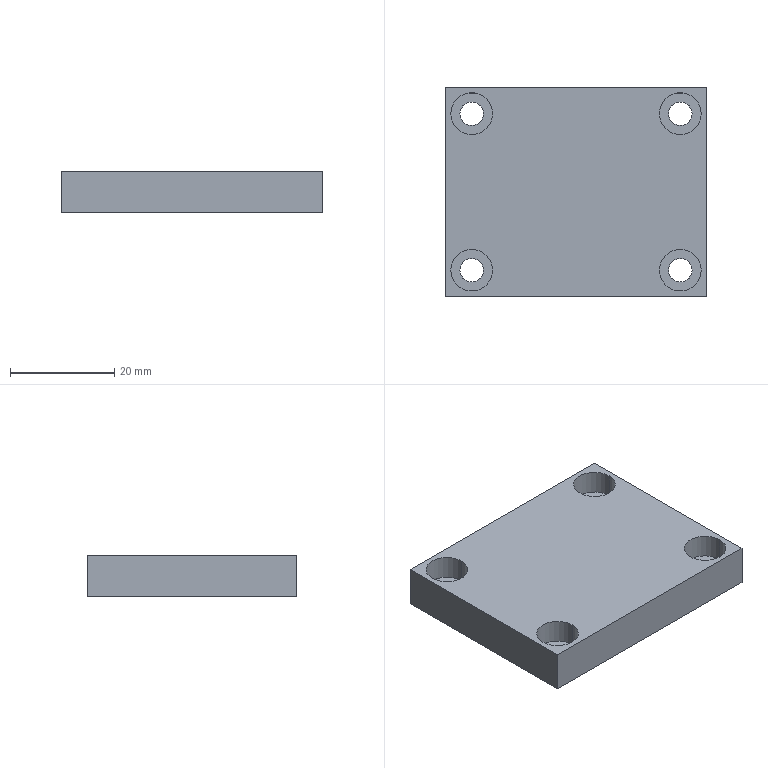Part | STEP file | X77-03306 | 1 solid | 26 faces | box 50 x 40 x 8 mm | volume 14859 mm3 | cylinder 16 | plane 10 | commonest cylinder face diameters 4.5 x8 8 x8
STEP:
#1=CARTESIAN_POINT('',(-1311.516,459.802,3.4));
#2=VERTEX_POINT('',#1);
#3=CARTESIAN_POINT('',(-1303.516,459.802,3.4));
#4=VERTEX_POINT('',#3);
#5=CARTESIAN_POINT('',(-1307.516,459.802,3.4));
#6=DIRECTION('',(0.,0.,1.));
#7=DIRECTION('',(1.,0.,0.));
#8=AXIS2_PLACEMENT_3D('',#5,#6,#7);
#9=CIRCLE('',#8,4.);
#10=EDGE_CURVE('',#2,#4,#9,.T.);
#11=ORIENTED_EDGE('',*,*,#10,.F.);
#12=CARTESIAN_POINT('',(-1311.516,459.802,8.));
#13=VERTEX_POINT('',#12);
#14=CARTESIAN_POINT('',(-1311.516,459.802,8.));
#15=DIRECTION('',(0.,0.,1.));
#16=VECTOR('',#15,1000.);
#17=LINE('',#14,#16);
#18=EDGE_CURVE('',#2,#13,#17,.T.);
#19=ORIENTED_EDGE('',*,*,#18,.T.);
#20=CARTESIAN_POINT('',(-1303.516,459.802,8.));
#21=VERTEX_POINT('',#20);
#22=CARTESIAN_POINT('',(-1307.516,459.802,8.));
#23=DIRECTION('',(0.,0.,1.));
#24=DIRECTION('',(1.,0.,0.));
#25=AXIS2_PLACEMENT_3D('',#22,#23,#24);
#26=CIRCLE('',#25,4.);
#27=EDGE_CURVE('',#13,#21,#26,.T.);
#28=ORIENTED_EDGE('',*,*,#27,.T.);
#29=CARTESIAN_POINT('',(-1303.516,459.802,8.));
#30=DIRECTION('',(0.,0.,1.));
#31=VECTOR('',#30,1000.);
#32=LINE('',#29,#31);
#33=EDGE_CURVE('',#4,#21,#32,.T.);
#34=ORIENTED_EDGE('',*,*,#33,.F.);
#35=EDGE_LOOP('',(#11,#19,#28,#34));
#36=FACE_OUTER_BOUND('',#35,.T.);
#37=CARTESIAN_POINT('',(-1307.516,459.802,8.));
#38=DIRECTION('',(0.,0.,1.));
#39=DIRECTION('',(1.,0.,0.));
#40=AXIS2_PLACEMENT_3D('',#37,#38,#39);
#41=CYLINDRICAL_SURFACE('',#40,4.);
#42=ADVANCED_FACE('',(#36),#41,.F.);
#43=CARTESIAN_POINT('',(-1309.766,459.802,0.));
#44=VERTEX_POINT('',#43);
#45=CARTESIAN_POINT('',(-1305.266,459.802,0.));
#46=VERTEX_POINT('',#45);
#47=CARTESIAN_POINT('',(-1307.516,459.802,0.));
#48=DIRECTION('',(0.,0.,1.));
#49=DIRECTION('',(1.,0.,0.));
#50=AXIS2_PLACEMENT_3D('',#47,#48,#49);
#51=CIRCLE('',#50,2.25);
#52=EDGE_CURVE('',#44,#46,#51,.T.);
#53=ORIENTED_EDGE('',*,*,#52,.F.);
#54=CARTESIAN_POINT('',(-1309.766,459.802,3.4));
#55=VERTEX_POINT('',#54);
#56=CARTESIAN_POINT('',(-1309.766,459.802,8.));
#57=DIRECTION('',(0.,0.,1.));
#58=VECTOR('',#57,1000.);
#59=LINE('',#56,#58);
#60=EDGE_CURVE('',#44,#55,#59,.T.);
#61=ORIENTED_EDGE('',*,*,#60,.T.);
#62=CARTESIAN_POINT('',(-1305.266,459.802,3.4));
#63=VERTEX_POINT('',#62);
#64=CARTESIAN_POINT('',(-1307.516,459.802,3.4));
#65=DIRECTION('',(0.,0.,1.));
#66=DIRECTION('',(1.,0.,0.));
#67=AXIS2_PLACEMENT_3D('',#64,#65,#66);
#68=CIRCLE('',#67,2.25);
#69=EDGE_CURVE('',#55,#63,#68,.T.);
#70=ORIENTED_EDGE('',*,*,#69,.T.);
#71=CARTESIAN_POINT('',(-1305.266,459.802,8.));
#72=DIRECTION('',(0.,0.,1.));
#73=VECTOR('',#72,1000.);
#74=LINE('',#71,#73);
#75=EDGE_CURVE('',#46,#63,#74,.T.);
#76=ORIENTED_EDGE('',*,*,#75,.F.);
#77=EDGE_LOOP('',(#53,#61,#70,#76));
#78=FACE_OUTER_BOUND('',#77,.T.);
#79=CARTESIAN_POINT('',(-1307.516,459.802,8.));
#80=DIRECTION('',(0.,0.,1.));
#81=DIRECTION('',(1.,0.,0.));
#82=AXIS2_PLACEMENT_3D('',#79,#80,#81);
#83=CYLINDRICAL_SURFACE('',#82,2.25);
#84=ADVANCED_FACE('',(#78),#83,.F.);
#85=CARTESIAN_POINT('',(-1311.516,429.802,3.4));
#86=VERTEX_POINT('',#85);
#87=CARTESIAN_POINT('',(-1303.516,429.802,3.4));
#88=VERTEX_POINT('',#87);
#89=CARTESIAN_POINT('',(-1307.516,429.802,3.4));
#90=DIRECTION('',(0.,0.,1.));
#91=DIRECTION('',(1.,0.,0.));
#92=AXIS2_PLACEMENT_3D('',#89,#90,#91);
#93=CIRCLE('',#92,4.);
#94=EDGE_CURVE('',#86,#88,#93,.T.);
#95=ORIENTED_EDGE('',*,*,#94,.F.);
#96=CARTESIAN_POINT('',(-1311.516,429.802,8.));
#97=VERTEX_POINT('',#96);
#98=CARTESIAN_POINT('',(-1311.516,429.802,8.));
#99=DIRECTION('',(0.,0.,1.));
#100=VECTOR('',#99,1000.);
#101=LINE('',#98,#100);
#102=EDGE_CURVE('',#86,#97,#101,.T.);
#103=ORIENTED_EDGE('',*,*,#102,.T.);
#104=CARTESIAN_POINT('',(-1303.516,429.802,8.));
#105=VERTEX_POINT('',#104);
#106=CARTESIAN_POINT('',(-1307.516,429.802,8.));
#107=DIRECTION('',(0.,0.,1.));
#108=DIRECTION('',(1.,0.,0.));
#109=AXIS2_PLACEMENT_3D('',#106,#107,#108);
#110=CIRCLE('',#109,4.);
#111=EDGE_CURVE('',#97,#105,#110,.T.);
#112=ORIENTED_EDGE('',*,*,#111,.T.);
#113=CARTESIAN_POINT('',(-1303.516,429.802,8.));
#114=DIRECTION('',(0.,0.,1.));
#115=VECTOR('',#114,1000.);
#116=LINE('',#113,#115);
#117=EDGE_CURVE('',#88,#105,#116,.T.);
#118=ORIENTED_EDGE('',*,*,#117,.F.);
#119=EDGE_LOOP('',(#95,#103,#112,#118));
#120=FACE_OUTER_BOUND('',#119,.T.);
#121=CARTESIAN_POINT('',(-1307.516,429.802,8.));
#122=DIRECTION('',(0.,0.,1.));
#123=DIRECTION('',(1.,0.,0.));
#124=AXIS2_PLACEMENT_3D('',#121,#122,#123);
#125=CYLINDRICAL_SURFACE('',#124,4.);
#126=ADVANCED_FACE('',(#120),#125,.F.);
#127=CARTESIAN_POINT('',(-1309.766,429.802,0.));
#128=VERTEX_POINT('',#127);
#129=CARTESIAN_POINT('',(-1305.266,429.802,0.));
#130=VERTEX_POINT('',#129);
#131=CARTESIAN_POINT('',(-1307.516,429.802,0.));
#132=DIRECTION('',(0.,0.,1.));
#133=DIRECTION('',(1.,0.,0.));
#134=AXIS2_PLACEMENT_3D('',#131,#132,#133);
#135=CIRCLE('',#134,2.25);
#136=EDGE_CURVE('',#128,#130,#135,.T.);
#137=ORIENTED_EDGE('',*,*,#136,.F.);
#138=CARTESIAN_POINT('',(-1309.766,429.802,3.4));
#139=VERTEX_POINT('',#138);
#140=CARTESIAN_POINT('',(-1309.766,429.802,8.));
#141=DIRECTION('',(0.,0.,1.));
#142=VECTOR('',#141,1000.);
#143=LINE('',#140,#142);
#144=EDGE_CURVE('',#128,#139,#143,.T.);
#145=ORIENTED_EDGE('',*,*,#144,.T.);
#146=CARTESIAN_POINT('',(-1305.266,429.802,3.4));
#147=VERTEX_POINT('',#146);
#148=CARTESIAN_POINT('',(-1307.516,429.802,3.4));
#149=DIRECTION('',(0.,0.,1.));
#150=DIRECTION('',(1.,0.,0.));
#151=AXIS2_PLACEMENT_3D('',#148,#149,#150);
#152=CIRCLE('',#151,2.25);
#153=EDGE_CURVE('',#139,#147,#152,.T.);
#154=ORIENTED_EDGE('',*,*,#153,.T.);
#155=CARTESIAN_POINT('',(-1305.266,429.802,8.));
#156=DIRECTION('',(0.,0.,1.));
#157=VECTOR('',#156,1000.);
#158=LINE('',#155,#157);
#159=EDGE_CURVE('',#130,#147,#158,.T.);
#160=ORIENTED_EDGE('',*,*,#159,.F.);
#161=EDGE_LOOP('',(#137,#145,#154,#160));
#162=FACE_OUTER_BOUND('',#161,.T.);
#163=CARTESIAN_POINT('',(-1307.516,429.802,8.));
#164=DIRECTION('',(0.,0.,1.));
#165=DIRECTION('',(1.,0.,0.));
#166=AXIS2_PLACEMENT_3D('',#163,#164,#165);
#167=CYLINDRICAL_SURFACE('',#166,2.25);
#168=ADVANCED_FACE('',(#162),#167,.F.);
#169=CARTESIAN_POINT('',(-1351.516,429.802,3.4));
#170=VERTEX_POINT('',#169);
#171=CARTESIAN_POINT('',(-1343.516,429.802,3.4));
#172=VERTEX_POINT('',#171);
#173=CARTESIAN_POINT('',(-1347.516,429.802,3.4));
#174=DIRECTION('',(0.,0.,1.));
#175=DIRECTION('',(1.,0.,0.));
#176=AXIS2_PLACEMENT_3D('',#173,#174,#175);
#177=CIRCLE('',#176,4.);
#178=EDGE_CURVE('',#170,#172,#177,.T.);
#179=ORIENTED_EDGE('',*,*,#178,.F.);
#180=CARTESIAN_POINT('',(-1351.516,429.802,8.));
#181=VERTEX_POINT('',#180);
#182=CARTESIAN_POINT('',(-1351.516,429.802,8.));
#183=DIRECTION('',(0.,0.,1.));
#184=VECTOR('',#183,1000.);
#185=LINE('',#182,#184);
#186=EDGE_CURVE('',#170,#181,#185,.T.);
#187=ORIENTED_EDGE('',*,*,#186,.T.);
#188=CARTESIAN_POINT('',(-1343.516,429.802,8.));
#189=VERTEX_POINT('',#188);
#190=CARTESIAN_POINT('',(-1347.516,429.802,8.));
#191=DIRECTION('',(0.,0.,1.));
#192=DIRECTION('',(1.,0.,0.));
#193=AXIS2_PLACEMENT_3D('',#190,#191,#192);
#194=CIRCLE('',#193,4.);
#195=EDGE_CURVE('',#181,#189,#194,.T.);
#196=ORIENTED_EDGE('',*,*,#195,.T.);
#197=CARTESIAN_POINT('',(-1343.516,429.802,8.));
#198=DIRECTION('',(0.,0.,1.));
#199=VECTOR('',#198,1000.);
#200=LINE('',#197,#199);
#201=EDGE_CURVE('',#172,#189,#200,.T.);
#202=ORIENTED_EDGE('',*,*,#201,.F.);
#203=EDGE_LOOP('',(#179,#187,#196,#202));
#204=FACE_OUTER_BOUND('',#203,.T.);
#205=CARTESIAN_POINT('',(-1347.516,429.802,8.));
#206=DIRECTION('',(0.,0.,1.));
#207=DIRECTION('',(1.,0.,0.));
#208=AXIS2_PLACEMENT_3D('',#205,#206,#207);
#209=CYLINDRICAL_SURFACE('',#208,4.);
#210=ADVANCED_FACE('',(#204),#209,.F.);
#211=CARTESIAN_POINT('',(-1349.766,429.802,0.));
#212=VERTEX_POINT('',#211);
#213=CARTESIAN_POINT('',(-1345.266,429.802,0.));
#214=VERTEX_POINT('',#213);
#215=CARTESIAN_POINT('',(-1347.516,429.802,0.));
#216=DIRECTION('',(0.,0.,1.));
#217=DIRECTION('',(1.,0.,0.));
#218=AXIS2_PLACEMENT_3D('',#215,#216,#217);
#219=CIRCLE('',#218,2.25);
#220=EDGE_CURVE('',#212,#214,#219,.T.);
#221=ORIENTED_EDGE('',*,*,#220,.F.);
#222=CARTESIAN_POINT('',(-1349.766,429.802,3.4));
#223=VERTEX_POINT('',#222);
#224=CARTESIAN_POINT('',(-1349.766,429.802,8.));
#225=DIRECTION('',(0.,0.,1.));
#226=VECTOR('',#225,1000.);
#227=LINE('',#224,#226);
#228=EDGE_CURVE('',#212,#223,#227,.T.);
#229=ORIENTED_EDGE('',*,*,#228,.T.);
#230=CARTESIAN_POINT('',(-1345.266,429.802,3.4));
#231=VERTEX_POINT('',#230);
#232=CARTESIAN_POINT('',(-1347.516,429.802,3.4));
#233=DIRECTION('',(0.,0.,1.));
#234=DIRECTION('',(1.,0.,0.));
#235=AXIS2_PLACEMENT_3D('',#232,#233,#234);
#236=CIRCLE('',#235,2.25);
#237=EDGE_CURVE('',#223,#231,#236,.T.);
#238=ORIENTED_EDGE('',*,*,#237,.T.);
#239=CARTESIAN_POINT('',(-1345.266,429.802,8.));
#240=DIRECTION('',(0.,0.,1.));
#241=VECTOR('',#240,1000.);
#242=LINE('',#239,#241);
#243=EDGE_CURVE('',#214,#231,#242,.T.);
#244=ORIENTED_EDGE('',*,*,#243,.F.);
#245=EDGE_LOOP('',(#221,#229,#238,#244));
#246=FACE_OUTER_BOUND('',#245,.T.);
#247=CARTESIAN_POINT('',(-1347.516,429.802,8.));
#248=DIRECTION('',(0.,0.,1.));
#249=DIRECTION('',(1.,0.,0.));
#250=AXIS2_PLACEMENT_3D('',#247,#248,#249);
#251=CYLINDRICAL_SURFACE('',#250,2.25);
#252=ADVANCED_FACE('',(#246),#251,.F.);
#253=CARTESIAN_POINT('',(-1351.516,459.802,3.4));
#254=VERTEX_POINT('',#253);
#255=CARTESIAN_POINT('',(-1343.516,459.802,3.4));
#256=VERTEX_POINT('',#255);
#257=CARTESIAN_POINT('',(-1347.516,459.802,3.4));
#258=DIRECTION('',(0.,0.,1.));
#259=DIRECTION('',(1.,0.,0.));
#260=AXIS2_PLACEMENT_3D('',#257,#258,#259);
#261=CIRCLE('',#260,4.);
#262=EDGE_CURVE('',#254,#256,#261,.T.);
#263=ORIENTED_EDGE('',*,*,#262,.F.);
#264=CARTESIAN_POINT('',(-1351.516,459.802,8.));
#265=VERTEX_POINT('',#264);
#266=CARTESIAN_POINT('',(-1351.516,459.802,8.));
#267=DIRECTION('',(0.,0.,1.));
#268=VECTOR('',#267,1000.);
#269=LINE('',#266,#268);
#270=EDGE_CURVE('',#254,#265,#269,.T.);
#271=ORIENTED_EDGE('',*,*,#270,.T.);
#272=CARTESIAN_POINT('',(-1343.516,459.802,8.));
#273=VERTEX_POINT('',#272);
#274=CARTESIAN_POINT('',(-1347.516,459.802,8.));
#275=DIRECTION('',(0.,0.,1.));
#276=DIRECTION('',(1.,0.,0.));
#277=AXIS2_PLACEMENT_3D('',#274,#275,#276);
#278=CIRCLE('',#277,4.);
#279=EDGE_CURVE('',#265,#273,#278,.T.);
#280=ORIENTED_EDGE('',*,*,#279,.T.);
#281=CARTESIAN_POINT('',(-1343.516,459.802,8.));
#282=DIRECTION('',(0.,0.,1.));
#283=VECTOR('',#282,1000.);
#284=LINE('',#281,#283);
#285=EDGE_CURVE('',#256,#273,#284,.T.);
#286=ORIENTED_EDGE('',*,*,#285,.F.);
#287=EDGE_LOOP('',(#263,#271,#280,#286));
#288=FACE_OUTER_BOUND('',#287,.T.);
#289=CARTESIAN_POINT('',(-1347.516,459.802,8.));
#290=DIRECTION('',(0.,0.,1.));
#291=DIRECTION('',(1.,0.,0.));
#292=AXIS2_PLACEMENT_3D('',#289,#290,#291);
#293=CYLINDRICAL_SURFACE('',#292,4.);
#294=ADVANCED_FACE('',(#288),#293,.F.);
#295=CARTESIAN_POINT('',(-1349.766,459.802,0.));
#296=VERTEX_POINT('',#295);
#297=CARTESIAN_POINT('',(-1345.266,459.802,0.));
#298=VERTEX_POINT('',#297);
#299=CARTESIAN_POINT('',(-1347.516,459.802,0.));
#300=DIRECTION('',(0.,0.,1.));
#301=DIRECTION('',(1.,0.,0.));
#302=AXIS2_PLACEMENT_3D('',#299,#300,#301);
#303=CIRCLE('',#302,2.25);
#304=EDGE_CURVE('',#296,#298,#303,.T.);
#305=ORIENTED_EDGE('',*,*,#304,.F.);
#306=CARTESIAN_POINT('',(-1349.766,459.802,3.4));
#307=VERTEX_POINT('',#306);
#308=CARTESIAN_POINT('',(-1349.766,459.802,8.));
#309=DIRECTION('',(0.,0.,1.));
#310=VECTOR('',#309,1000.);
#311=LINE('',#308,#310);
#312=EDGE_CURVE('',#296,#307,#311,.T.);
#313=ORIENTED_EDGE('',*,*,#312,.T.);
#314=CARTESIAN_POINT('',(-1345.266,459.802,3.4));
#315=VERTEX_POINT('',#314);
#316=CARTESIAN_POINT('',(-1347.516,459.802,3.4));
#317=DIRECTION('',(0.,0.,1.));
#318=DIRECTION('',(1.,0.,0.));
#319=AXIS2_PLACEMENT_3D('',#316,#317,#318);
#320=CIRCLE('',#319,2.25);
#321=EDGE_CURVE('',#307,#315,#320,.T.);
#322=ORIENTED_EDGE('',*,*,#321,.T.);
#323=CARTESIAN_POINT('',(-1345.266,459.802,8.));
#324=DIRECTION('',(0.,0.,1.));
#325=VECTOR('',#324,1000.);
#326=LINE('',#323,#325);
#327=EDGE_CURVE('',#298,#315,#326,.T.);
#328=ORIENTED_EDGE('',*,*,#327,.F.);
#329=EDGE_LOOP('',(#305,#313,#322,#328));
#330=FACE_OUTER_BOUND('',#329,.T.);
#331=CARTESIAN_POINT('',(-1347.516,459.802,8.));
#332=DIRECTION('',(0.,0.,1.));
#333=DIRECTION('',(1.,0.,0.));
#334=AXIS2_PLACEMENT_3D('',#331,#332,#333);
#335=CYLINDRICAL_SURFACE('',#334,2.25);
#336=ADVANCED_FACE('',(#330),#335,.F.);
#337=CARTESIAN_POINT('',(-1352.516,464.802,0.));
#338=VERTEX_POINT('',#337);
#339=CARTESIAN_POINT('',(-1352.516,424.802,0.));
#340=VERTEX_POINT('',#339);
#341=CARTESIAN_POINT('',(-1352.516,464.802,0.));
#342=DIRECTION('',(0.,-1.,0.));
#343=VECTOR('',#342,1000.);
#344=LINE('',#341,#343);
#345=EDGE_CURVE('',#338,#340,#344,.T.);
#346=ORIENTED_EDGE('',*,*,#345,.T.);
#347=CARTESIAN_POINT('',(-1352.516,424.802,8.));
#348=VERTEX_POINT('',#347);
#349=CARTESIAN_POINT('',(-1352.516,424.802,8.));
#350=DIRECTION('',(0.,0.,-1.));
#351=VECTOR('',#350,1000.);
#352=LINE('',#349,#351);
#353=EDGE_CURVE('',#348,#340,#352,.T.);
#354=ORIENTED_EDGE('',*,*,#353,.F.);
#355=CARTESIAN_POINT('',(-1352.516,464.802,8.));
#356=VERTEX_POINT('',#355);
#357=CARTESIAN_POINT('',(-1352.516,464.802,8.));
#358=DIRECTION('',(0.,-1.,0.));
#359=VECTOR('',#358,1000.);
#360=LINE('',#357,#359);
#361=EDGE_CURVE('',#356,#348,#360,.T.);
#362=ORIENTED_EDGE('',*,*,#361,.F.);
#363=CARTESIAN_POINT('',(-1352.516,464.802,8.));
#364=DIRECTION('',(0.,0.,-1.));
#365=VECTOR('',#364,1000.);
#366=LINE('',#363,#365);
#367=EDGE_CURVE('',#356,#338,#366,.T.);
#368=ORIENTED_EDGE('',*,*,#367,.T.);
#369=EDGE_LOOP('',(#346,#354,#362,#368));
#370=FACE_OUTER_BOUND('',#369,.T.);
#371=CARTESIAN_POINT('',(-1352.516,464.802,8.));
#372=DIRECTION('',(1.,0.,0.));
#373=DIRECTION('',(0.,0.,-1.));
#374=AXIS2_PLACEMENT_3D('',#371,#372,#373);
#375=PLANE('',#374);
#376=ADVANCED_FACE('',(#370),#375,.F.);
#377=CARTESIAN_POINT('',(-1302.516,424.802,0.));
#378=VERTEX_POINT('',#377);
#379=CARTESIAN_POINT('',(-1352.516,424.802,0.));
#380=DIRECTION('',(1.,0.,0.));
#381=VECTOR('',#380,1000.);
#382=LINE('',#379,#381);
#383=EDGE_CURVE('',#340,#378,#382,.T.);
#384=ORIENTED_EDGE('',*,*,#383,.T.);
#385=CARTESIAN_POINT('',(-1302.516,424.802,8.));
#386=VERTEX_POINT('',#385);
#387=CARTESIAN_POINT('',(-1302.516,424.802,8.));
#388=DIRECTION('',(0.,0.,-1.));
#389=VECTOR('',#388,1000.);
#390=LINE('',#387,#389);
#391=EDGE_CURVE('',#386,#378,#390,.T.);
#392=ORIENTED_EDGE('',*,*,#391,.F.);
#393=CARTESIAN_POINT('',(-1352.516,424.802,8.));
#394=DIRECTION('',(1.,0.,0.));
#395=VECTOR('',#394,1000.);
#396=LINE('',#393,#395);
#397=EDGE_CURVE('',#348,#386,#396,.T.);
#398=ORIENTED_EDGE('',*,*,#397,.F.);
#399=ORIENTED_EDGE('',*,*,#353,.T.);
#400=EDGE_LOOP('',(#384,#392,#398,#399));
#401=FACE_OUTER_BOUND('',#400,.T.);
#402=CARTESIAN_POINT('',(-1352.516,424.802,8.));
#403=DIRECTION('',(0.,1.,0.));
#404=DIRECTION('',(0.,0.,1.));
#405=AXIS2_PLACEMENT_3D('',#402,#403,#404);
#406=PLANE('',#405);
#407=ADVANCED_FACE('',(#401),#406,.F.);
#408=CARTESIAN_POINT('',(-1302.516,464.802,0.));
#409=VERTEX_POINT('',#408);
#410=CARTESIAN_POINT('',(-1302.516,464.802,0.));
#411=DIRECTION('',(0.,1.,0.));
#412=VECTOR('',#411,1000.);
#413=LINE('',#410,#412);
#414=EDGE_CURVE('',#378,#409,#413,.T.);
#415=ORIENTED_EDGE('',*,*,#414,.T.);
#416=CARTESIAN_POINT('',(-1302.516,464.802,8.));
#417=VERTEX_POINT('',#416);
#418=CARTESIAN_POINT('',(-1302.516,464.802,8.));
#419=DIRECTION('',(0.,0.,-1.));
#420=VECTOR('',#419,1000.);
#421=LINE('',#418,#420);
#422=EDGE_CURVE('',#417,#409,#421,.T.);
#423=ORIENTED_EDGE('',*,*,#422,.F.);
#424=CARTESIAN_POINT('',(-1302.516,464.802,8.));
#425=DIRECTION('',(0.,1.,0.));
#426=VECTOR('',#425,1000.);
#427=LINE('',#424,#426);
#428=EDGE_CURVE('',#386,#417,#427,.T.);
#429=ORIENTED_EDGE('',*,*,#428,.F.);
#430=ORIENTED_EDGE('',*,*,#391,.T.);
#431=EDGE_LOOP('',(#415,#423,#429,#430));
#432=FACE_OUTER_BOUND('',#431,.T.);
#433=CARTESIAN_POINT('',(-1302.516,464.802,8.));
#434=DIRECTION('',(-1.,0.,0.));
#435=DIRECTION('',(0.,0.,1.));
#436=AXIS2_PLACEMENT_3D('',#433,#434,#435);
#437=PLANE('',#436);
#438=ADVANCED_FACE('',(#432),#437,.F.);
#439=CARTESIAN_POINT('',(-1352.516,464.802,0.));
#440=DIRECTION('',(-1.,0.,0.));
#441=VECTOR('',#440,1000.);
#442=LINE('',#439,#441);
#443=EDGE_CURVE('',#409,#338,#442,.T.);
#444=ORIENTED_EDGE('',*,*,#443,.T.);
#445=ORIENTED_EDGE('',*,*,#367,.F.);
#446=CARTESIAN_POINT('',(-1352.516,464.802,8.));
#447=DIRECTION('',(-1.,0.,0.));
#448=VECTOR('',#447,1000.);
#449=LINE('',#446,#448);
#450=EDGE_CURVE('',#417,#356,#449,.T.);
#451=ORIENTED_EDGE('',*,*,#450,.F.);
#452=ORIENTED_EDGE('',*,*,#422,.T.);
#453=EDGE_LOOP('',(#444,#445,#451,#452));
#454=FACE_OUTER_BOUND('',#453,.T.);
#455=CARTESIAN_POINT('',(-1352.516,464.802,8.));
#456=DIRECTION('',(0.,-1.,0.));
#457=DIRECTION('',(0.,0.,-1.));
#458=AXIS2_PLACEMENT_3D('',#455,#456,#457);
#459=PLANE('',#458);
#460=ADVANCED_FACE('',(#454),#459,.F.);
#461=CARTESIAN_POINT('',(-1307.516,459.802,8.));
#462=DIRECTION('',(0.,0.,1.));
#463=DIRECTION('',(1.,0.,0.));
#464=AXIS2_PLACEMENT_3D('',#461,#462,#463);
#465=CIRCLE('',#464,4.);
#466=EDGE_CURVE('',#21,#13,#465,.T.);
#467=ORIENTED_EDGE('',*,*,#466,.F.);
#468=ORIENTED_EDGE('',*,*,#27,.F.);
#469=EDGE_LOOP('',(#467,#468));
#470=FACE_BOUND('',#469,.T.);
#471=CARTESIAN_POINT('',(-1307.516,429.802,8.));
#472=DIRECTION('',(0.,0.,1.));
#473=DIRECTION('',(1.,0.,0.));
#474=AXIS2_PLACEMENT_3D('',#471,#472,#473);
#475=CIRCLE('',#474,4.);
#476=EDGE_CURVE('',#105,#97,#475,.T.);
#477=ORIENTED_EDGE('',*,*,#476,.F.);
#478=ORIENTED_EDGE('',*,*,#111,.F.);
#479=EDGE_LOOP('',(#477,#478));
#480=FACE_BOUND('',#479,.T.);
#481=CARTESIAN_POINT('',(-1347.516,429.802,8.));
#482=DIRECTION('',(0.,0.,1.));
#483=DIRECTION('',(1.,0.,0.));
#484=AXIS2_PLACEMENT_3D('',#481,#482,#483);
#485=CIRCLE('',#484,4.);
#486=EDGE_CURVE('',#189,#181,#485,.T.);
#487=ORIENTED_EDGE('',*,*,#486,.F.);
#488=ORIENTED_EDGE('',*,*,#195,.F.);
#489=EDGE_LOOP('',(#487,#488));
#490=FACE_BOUND('',#489,.T.);
#491=CARTESIAN_POINT('',(-1347.516,459.802,8.));
#492=DIRECTION('',(0.,0.,1.));
#493=DIRECTION('',(1.,0.,0.));
#494=AXIS2_PLACEMENT_3D('',#491,#492,#493);
#495=CIRCLE('',#494,4.);
#496=EDGE_CURVE('',#273,#265,#495,.T.);
#497=ORIENTED_EDGE('',*,*,#496,.F.);
#498=ORIENTED_EDGE('',*,*,#279,.F.);
#499=EDGE_LOOP('',(#497,#498));
#500=FACE_BOUND('',#499,.T.);
#501=ORIENTED_EDGE('',*,*,#361,.T.);
#502=ORIENTED_EDGE('',*,*,#397,.T.);
#503=ORIENTED_EDGE('',*,*,#428,.T.);
#504=ORIENTED_EDGE('',*,*,#450,.T.);
#505=EDGE_LOOP('',(#501,#502,#503,#504));
#506=FACE_OUTER_BOUND('',#505,.T.);
#507=CARTESIAN_POINT('',(-1352.516,424.802,8.));
#508=DIRECTION('',(0.,0.,1.));
#509=DIRECTION('',(1.,0.,0.));
#510=AXIS2_PLACEMENT_3D('',#507,#508,#509);
#511=PLANE('',#510);
#512=ADVANCED_FACE('',(#470,#480,#490,#500,#506),#511,.T.);
#513=CARTESIAN_POINT('',(-1307.516,459.802,0.));
#514=DIRECTION('',(0.,0.,1.));
#515=DIRECTION('',(1.,0.,0.));
#516=AXIS2_PLACEMENT_3D('',#513,#514,#515);
#517=CIRCLE('',#516,2.25);
#518=EDGE_CURVE('',#46,#44,#517,.T.);
#519=ORIENTED_EDGE('',*,*,#518,.T.);
#520=ORIENTED_EDGE('',*,*,#52,.T.);
#521=EDGE_LOOP('',(#519,#520));
#522=FACE_BOUND('',#521,.T.);
#523=CARTESIAN_POINT('',(-1307.516,429.802,0.));
#524=DIRECTION('',(0.,0.,1.));
#525=DIRECTION('',(1.,0.,0.));
#526=AXIS2_PLACEMENT_3D('',#523,#524,#525);
#527=CIRCLE('',#526,2.25);
#528=EDGE_CURVE('',#130,#128,#527,.T.);
#529=ORIENTED_EDGE('',*,*,#528,.T.);
#530=ORIENTED_EDGE('',*,*,#136,.T.);
#531=EDGE_LOOP('',(#529,#530));
#532=FACE_BOUND('',#531,.T.);
#533=CARTESIAN_POINT('',(-1347.516,429.802,0.));
#534=DIRECTION('',(0.,0.,1.));
#535=DIRECTION('',(1.,0.,0.));
#536=AXIS2_PLACEMENT_3D('',#533,#534,#535);
#537=CIRCLE('',#536,2.25);
#538=EDGE_CURVE('',#214,#212,#537,.T.);
#539=ORIENTED_EDGE('',*,*,#538,.T.);
#540=ORIENTED_EDGE('',*,*,#220,.T.);
#541=EDGE_LOOP('',(#539,#540));
#542=FACE_BOUND('',#541,.T.);
#543=CARTESIAN_POINT('',(-1347.516,459.802,0.));
#544=DIRECTION('',(0.,0.,1.));
#545=DIRECTION('',(1.,0.,0.));
#546=AXIS2_PLACEMENT_3D('',#543,#544,#545);
#547=CIRCLE('',#546,2.25);
#548=EDGE_CURVE('',#298,#296,#547,.T.);
#549=ORIENTED_EDGE('',*,*,#548,.T.);
#550=ORIENTED_EDGE('',*,*,#304,.T.);
#551=EDGE_LOOP('',(#549,#550));
#552=FACE_BOUND('',#551,.T.);
#553=ORIENTED_EDGE('',*,*,#345,.F.);
#554=ORIENTED_EDGE('',*,*,#443,.F.);
#555=ORIENTED_EDGE('',*,*,#414,.F.);
#556=ORIENTED_EDGE('',*,*,#383,.F.);
#557=EDGE_LOOP('',(#553,#554,#555,#556));
#558=FACE_OUTER_BOUND('',#557,.T.);
#559=CARTESIAN_POINT('',(-1352.516,424.802,0.));
#560=DIRECTION('',(0.,0.,1.));
#561=DIRECTION('',(1.,0.,0.));
#562=AXIS2_PLACEMENT_3D('',#559,#560,#561);
#563=PLANE('',#562);
#564=ADVANCED_FACE('',(#522,#532,#542,#552,#558),#563,.F.);
#565=ORIENTED_EDGE('',*,*,#312,.F.);
#566=ORIENTED_EDGE('',*,*,#548,.F.);
#567=ORIENTED_EDGE('',*,*,#327,.T.);
#568=CARTESIAN_POINT('',(-1347.516,459.802,3.4));
#569=DIRECTION('',(0.,0.,1.));
#570=DIRECTION('',(1.,0.,0.));
#571=AXIS2_PLACEMENT_3D('',#568,#569,#570);
#572=CIRCLE('',#571,2.25);
#573=EDGE_CURVE('',#315,#307,#572,.T.);
#574=ORIENTED_EDGE('',*,*,#573,.T.);
#575=EDGE_LOOP('',(#565,#566,#567,#574));
#576=FACE_OUTER_BOUND('',#575,.T.);
#577=CARTESIAN_POINT('',(-1347.516,459.802,8.));
#578=DIRECTION('',(0.,0.,1.));
#579=DIRECTION('',(1.,0.,0.));
#580=AXIS2_PLACEMENT_3D('',#577,#578,#579);
#581=CYLINDRICAL_SURFACE('',#580,2.25);
#582=ADVANCED_FACE('',(#576),#581,.F.);
#583=ORIENTED_EDGE('',*,*,#573,.F.);
#584=ORIENTED_EDGE('',*,*,#321,.F.);
#585=EDGE_LOOP('',(#583,#584));
#586=FACE_BOUND('',#585,.T.);
#587=CARTESIAN_POINT('',(-1347.516,459.802,3.4));
#588=DIRECTION('',(0.,0.,1.));
#589=DIRECTION('',(1.,0.,0.));
#590=AXIS2_PLACEMENT_3D('',#587,#588,#589);
#591=CIRCLE('',#590,4.);
#592=EDGE_CURVE('',#256,#254,#591,.T.);
#593=ORIENTED_EDGE('',*,*,#592,.T.);
#594=ORIENTED_EDGE('',*,*,#262,.T.);
#595=EDGE_LOOP('',(#593,#594));
#596=FACE_OUTER_BOUND('',#595,.T.);
#597=CARTESIAN_POINT('',(-1345.266,459.802,3.4));
#598=DIRECTION('',(0.,0.,-1.));
#599=DIRECTION('',(-1.,0.,0.));
#600=AXIS2_PLACEMENT_3D('',#597,#598,#599);
#601=PLANE('',#600);
#602=ADVANCED_FACE('',(#586,#596),#601,.F.);
#603=ORIENTED_EDGE('',*,*,#270,.F.);
#604=ORIENTED_EDGE('',*,*,#592,.F.);
#605=ORIENTED_EDGE('',*,*,#285,.T.);
#606=ORIENTED_EDGE('',*,*,#496,.T.);
#607=EDGE_LOOP('',(#603,#604,#605,#606));
#608=FACE_OUTER_BOUND('',#607,.T.);
#609=CARTESIAN_POINT('',(-1347.516,459.802,8.));
#610=DIRECTION('',(0.,0.,1.));
#611=DIRECTION('',(1.,0.,0.));
#612=AXIS2_PLACEMENT_3D('',#609,#610,#611);
#613=CYLINDRICAL_SURFACE('',#612,4.);
#614=ADVANCED_FACE('',(#608),#613,.F.);
#615=ORIENTED_EDGE('',*,*,#228,.F.);
#616=ORIENTED_EDGE('',*,*,#538,.F.);
#617=ORIENTED_EDGE('',*,*,#243,.T.);
#618=CARTESIAN_POINT('',(-1347.516,429.802,3.4));
#619=DIRECTION('',(0.,0.,1.));
#620=DIRECTION('',(1.,0.,0.));
#621=AXIS2_PLACEMENT_3D('',#618,#619,#620);
#622=CIRCLE('',#621,2.25);
#623=EDGE_CURVE('',#231,#223,#622,.T.);
#624=ORIENTED_EDGE('',*,*,#623,.T.);
#625=EDGE_LOOP('',(#615,#616,#617,#624));
#626=FACE_OUTER_BOUND('',#625,.T.);
#627=CARTESIAN_POINT('',(-1347.516,429.802,8.));
#628=DIRECTION('',(0.,0.,1.));
#629=DIRECTION('',(1.,0.,0.));
#630=AXIS2_PLACEMENT_3D('',#627,#628,#629);
#631=CYLINDRICAL_SURFACE('',#630,2.25);
#632=ADVANCED_FACE('',(#626),#631,.F.);
#633=ORIENTED_EDGE('',*,*,#623,.F.);
#634=ORIENTED_EDGE('',*,*,#237,.F.);
#635=EDGE_LOOP('',(#633,#634));
#636=FACE_BOUND('',#635,.T.);
#637=CARTESIAN_POINT('',(-1347.516,429.802,3.4));
#638=DIRECTION('',(0.,0.,1.));
#639=DIRECTION('',(1.,0.,0.));
#640=AXIS2_PLACEMENT_3D('',#637,#638,#639);
#641=CIRCLE('',#640,4.);
#642=EDGE_CURVE('',#172,#170,#641,.T.);
#643=ORIENTED_EDGE('',*,*,#642,.T.);
#644=ORIENTED_EDGE('',*,*,#178,.T.);
#645=EDGE_LOOP('',(#643,#644));
#646=FACE_OUTER_BOUND('',#645,.T.);
#647=CARTESIAN_POINT('',(-1345.266,429.802,3.4));
#648=DIRECTION('',(0.,0.,-1.));
#649=DIRECTION('',(-1.,0.,0.));
#650=AXIS2_PLACEMENT_3D('',#647,#648,#649);
#651=PLANE('',#650);
#652=ADVANCED_FACE('',(#636,#646),#651,.F.);
#653=ORIENTED_EDGE('',*,*,#186,.F.);
#654=ORIENTED_EDGE('',*,*,#642,.F.);
#655=ORIENTED_EDGE('',*,*,#201,.T.);
#656=ORIENTED_EDGE('',*,*,#486,.T.);
#657=EDGE_LOOP('',(#653,#654,#655,#656));
#658=FACE_OUTER_BOUND('',#657,.T.);
#659=CARTESIAN_POINT('',(-1347.516,429.802,8.));
#660=DIRECTION('',(0.,0.,1.));
#661=DIRECTION('',(1.,0.,0.));
#662=AXIS2_PLACEMENT_3D('',#659,#660,#661);
#663=CYLINDRICAL_SURFACE('',#662,4.);
#664=ADVANCED_FACE('',(#658),#663,.F.);
#665=ORIENTED_EDGE('',*,*,#144,.F.);
#666=ORIENTED_EDGE('',*,*,#528,.F.);
#667=ORIENTED_EDGE('',*,*,#159,.T.);
#668=CARTESIAN_POINT('',(-1307.516,429.802,3.4));
#669=DIRECTION('',(0.,0.,1.));
#670=DIRECTION('',(1.,0.,0.));
#671=AXIS2_PLACEMENT_3D('',#668,#669,#670);
#672=CIRCLE('',#671,2.25);
#673=EDGE_CURVE('',#147,#139,#672,.T.);
#674=ORIENTED_EDGE('',*,*,#673,.T.);
#675=EDGE_LOOP('',(#665,#666,#667,#674));
#676=FACE_OUTER_BOUND('',#675,.T.);
#677=CARTESIAN_POINT('',(-1307.516,429.802,8.));
#678=DIRECTION('',(0.,0.,1.));
#679=DIRECTION('',(1.,0.,0.));
#680=AXIS2_PLACEMENT_3D('',#677,#678,#679);
#681=CYLINDRICAL_SURFACE('',#680,2.25);
#682=ADVANCED_FACE('',(#676),#681,.F.);
#683=ORIENTED_EDGE('',*,*,#673,.F.);
#684=ORIENTED_EDGE('',*,*,#153,.F.);
#685=EDGE_LOOP('',(#683,#684));
#686=FACE_BOUND('',#685,.T.);
#687=CARTESIAN_POINT('',(-1307.516,429.802,3.4));
#688=DIRECTION('',(0.,0.,1.));
#689=DIRECTION('',(1.,0.,0.));
#690=AXIS2_PLACEMENT_3D('',#687,#688,#689);
#691=CIRCLE('',#690,4.);
#692=EDGE_CURVE('',#88,#86,#691,.T.);
#693=ORIENTED_EDGE('',*,*,#692,.T.);
#694=ORIENTED_EDGE('',*,*,#94,.T.);
#695=EDGE_LOOP('',(#693,#694));
#696=FACE_OUTER_BOUND('',#695,.T.);
#697=CARTESIAN_POINT('',(-1305.266,429.802,3.4));
#698=DIRECTION('',(0.,0.,-1.));
#699=DIRECTION('',(-1.,0.,0.));
#700=AXIS2_PLACEMENT_3D('',#697,#698,#699);
#701=PLANE('',#700);
#702=ADVANCED_FACE('',(#686,#696),#701,.F.);
#703=ORIENTED_EDGE('',*,*,#102,.F.);
#704=ORIENTED_EDGE('',*,*,#692,.F.);
#705=ORIENTED_EDGE('',*,*,#117,.T.);
#706=ORIENTED_EDGE('',*,*,#476,.T.);
#707=EDGE_LOOP('',(#703,#704,#705,#706));
#708=FACE_OUTER_BOUND('',#707,.T.);
#709=CARTESIAN_POINT('',(-1307.516,429.802,8.));
#710=DIRECTION('',(0.,0.,1.));
#711=DIRECTION('',(1.,0.,0.));
#712=AXIS2_PLACEMENT_3D('',#709,#710,#711);
#713=CYLINDRICAL_SURFACE('',#712,4.);
#714=ADVANCED_FACE('',(#708),#713,.F.);
#715=ORIENTED_EDGE('',*,*,#60,.F.);
#716=ORIENTED_EDGE('',*,*,#518,.F.);
#717=ORIENTED_EDGE('',*,*,#75,.T.);
#718=CARTESIAN_POINT('',(-1307.516,459.802,3.4));
#719=DIRECTION('',(0.,0.,1.));
#720=DIRECTION('',(1.,0.,0.));
#721=AXIS2_PLACEMENT_3D('',#718,#719,#720);
#722=CIRCLE('',#721,2.25);
#723=EDGE_CURVE('',#63,#55,#722,.T.);
#724=ORIENTED_EDGE('',*,*,#723,.T.);
#725=EDGE_LOOP('',(#715,#716,#717,#724));
#726=FACE_OUTER_BOUND('',#725,.T.);
#727=CARTESIAN_POINT('',(-1307.516,459.802,8.));
#728=DIRECTION('',(0.,0.,1.));
#729=DIRECTION('',(1.,0.,0.));
#730=AXIS2_PLACEMENT_3D('',#727,#728,#729);
#731=CYLINDRICAL_SURFACE('',#730,2.25);
#732=ADVANCED_FACE('',(#726),#731,.F.);
#733=ORIENTED_EDGE('',*,*,#723,.F.);
#734=ORIENTED_EDGE('',*,*,#69,.F.);
#735=EDGE_LOOP('',(#733,#734));
#736=FACE_BOUND('',#735,.T.);
#737=CARTESIAN_POINT('',(-1307.516,459.802,3.4));
#738=DIRECTION('',(0.,0.,1.));
#739=DIRECTION('',(1.,0.,0.));
#740=AXIS2_PLACEMENT_3D('',#737,#738,#739);
#741=CIRCLE('',#740,4.);
#742=EDGE_CURVE('',#4,#2,#741,.T.);
#743=ORIENTED_EDGE('',*,*,#742,.T.);
#744=ORIENTED_EDGE('',*,*,#10,.T.);
#745=EDGE_LOOP('',(#743,#744));
#746=FACE_OUTER_BOUND('',#745,.T.);
#747=CARTESIAN_POINT('',(-1305.266,459.802,3.4));
#748=DIRECTION('',(0.,0.,-1.));
#749=DIRECTION('',(-1.,0.,0.));
#750=AXIS2_PLACEMENT_3D('',#747,#748,#749);
#751=PLANE('',#750);
#752=ADVANCED_FACE('',(#736,#746),#751,.F.);
#753=ORIENTED_EDGE('',*,*,#18,.F.);
#754=ORIENTED_EDGE('',*,*,#742,.F.);
#755=ORIENTED_EDGE('',*,*,#33,.T.);
#756=ORIENTED_EDGE('',*,*,#466,.T.);
#757=EDGE_LOOP('',(#753,#754,#755,#756));
#758=FACE_OUTER_BOUND('',#757,.T.);
#759=CARTESIAN_POINT('',(-1307.516,459.802,8.));
#760=DIRECTION('',(0.,0.,1.));
#761=DIRECTION('',(1.,0.,0.));
#762=AXIS2_PLACEMENT_3D('',#759,#760,#761);
#763=CYLINDRICAL_SURFACE('',#762,4.);
#764=ADVANCED_FACE('',(#758),#763,.F.);
#765=CLOSED_SHELL('',(#42,#84,#126,#168,#210,#252,#294,#336,#376,#407,#438,#460,#512,#564,#582,#602,#614,#632,#652,#664,#682,#702,#714,#732,#752,#764));
#766=MANIFOLD_SOLID_BREP('',#765);
#767=CARTESIAN_POINT('',(0.,0.,0.));
#768=DIRECTION('',(0.,0.,1.));
#769=DIRECTION('',(1.,0.,0.));
#770=AXIS2_PLACEMENT_3D('',#767,#768,#769);
#771=(LENGTH_UNIT()NAMED_UNIT(*)SI_UNIT(.MILLI.,.METRE.));
#772=UNCERTAINTY_MEASURE_WITH_UNIT(LENGTH_MEASURE(0.00001),#771,'','');
#773=(NAMED_UNIT(*)PLANE_ANGLE_UNIT()SI_UNIT($,.RADIAN.));
#774=(NAMED_UNIT(*)SI_UNIT($,.STERADIAN.)SOLID_ANGLE_UNIT());
#775=(GEOMETRIC_REPRESENTATION_CONTEXT(3)GLOBAL_UNCERTAINTY_ASSIGNED_CONTEXT((#772))GLOBAL_UNIT_ASSIGNED_CONTEXT((#771,#773,#774))REPRESENTATION_CONTEXT('',''));
#776=ADVANCED_BREP_SHAPE_REPRESENTATION('',(#766,#770),#775);